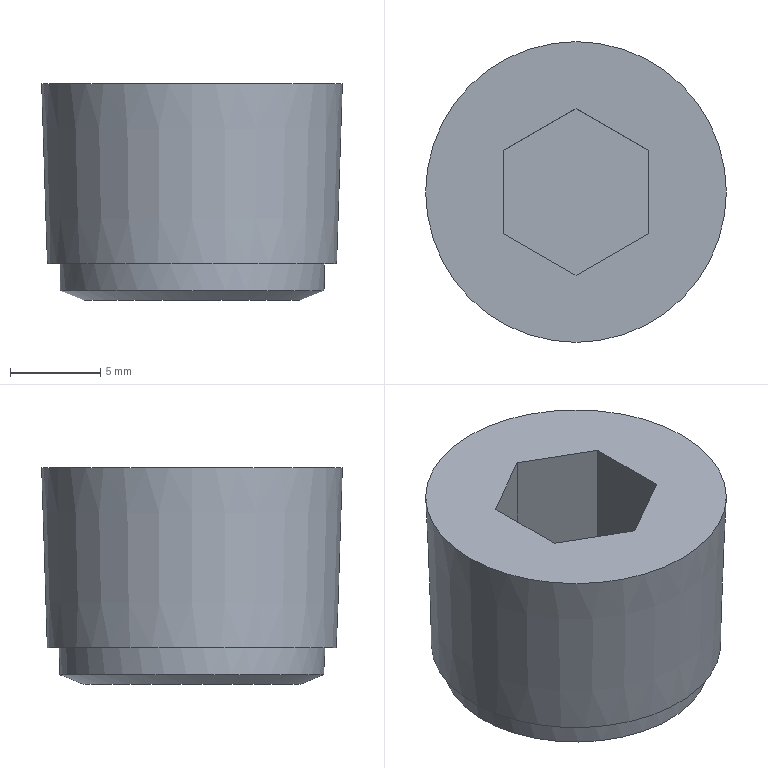Part | STEP file | SOLID | 1 solid | 13 faces | box 16.662 x 16.662 x 12.01 mm | volume 2091 mm3 | plane 10 | cone 3
STEP:
#1=CARTESIAN_POINT('',(0.,0.,0.));
#2=DIRECTION('',(0.,0.,1.));
#3=DIRECTION('',(1.,0.,0.));
#4=AXIS2_PLACEMENT_3D('',#1,#2,#3);
#5=CARTESIAN_POINT('',(0.,8.331,0.));
#6=VERTEX_POINT('',#5);
#7=CARTESIAN_POINT('',(0.,0.,0.));
#8=DIRECTION('',(0.,0.,1.));
#9=DIRECTION('',(0.,1.,0.));
#10=AXIS2_PLACEMENT_3D('',#7,#8,#9);
#11=CIRCLE('',#10,8.331);
#12=CARTESIAN_POINT('',(0.,0.,0.));
#13=DIRECTION('',(0.,0.,1.));
#14=DIRECTION('',(0.,1.,0.));
#15=AXIS2_PLACEMENT_3D('',#12,#13,#14);
#16=PLANE('',#15);
#17=CARTESIAN_POINT('',(0.,0.));
#18=DIRECTION('',(1.,0.));
#19=AXIS2_PLACEMENT_2D('',#17,#18);
#20=CIRCLE('',#19,8.331);
#21=(GEOMETRIC_REPRESENTATION_CONTEXT(2)PARAMETRIC_REPRESENTATION_CONTEXT()REPRESENTATION_CONTEXT('',''));
#22=DEFINITIONAL_REPRESENTATION('',(#20),#21);
#23=PCURVE('',#16,#22);
#24=CARTESIAN_POINT('',(0.,0.,-9.995));
#25=DIRECTION('',(0.,0.,1.));
#26=DIRECTION('',(0.,1.,0.));
#27=AXIS2_PLACEMENT_3D('',#24,#25,#26);
#28=CONICAL_SURFACE('',#27,8.017,0.03142);
#29=CARTESIAN_POINT('',(0.,9.995));
#30=DIRECTION('',(1.,0.));
#31=VECTOR('',#30,1.);
#32=LINE('',#29,#31);
#33=(GEOMETRIC_REPRESENTATION_CONTEXT(2)PARAMETRIC_REPRESENTATION_CONTEXT()REPRESENTATION_CONTEXT('',''));
#34=DEFINITIONAL_REPRESENTATION('',(#32),#33);
#35=PCURVE('',#28,#34);
#36=SURFACE_CURVE('',#11,(#23,#35),.PCURVE_S1.);
#37=EDGE_CURVE('',#6,#6,#36,.T.);
#38=ORIENTED_EDGE('',*,*,#37,.T.);
#39=EDGE_LOOP('',(#38));
#40=FACE_BOUND('',#39,.T.);
#41=CARTESIAN_POINT('',(-4.,-2.309,0.));
#42=VERTEX_POINT('',#41);
#43=CARTESIAN_POINT('',(-4.,2.309,0.));
#44=VERTEX_POINT('',#43);
#45=CARTESIAN_POINT('',(-4.,0.,0.));
#46=DIRECTION('',(0.,1.,0.));
#47=VECTOR('',#46,1.);
#48=LINE('',#45,#47);
#49=CARTESIAN_POINT('',(0.,4.));
#50=DIRECTION('',(1.,0.));
#51=VECTOR('',#50,1.);
#52=LINE('',#49,#51);
#53=(GEOMETRIC_REPRESENTATION_CONTEXT(2)PARAMETRIC_REPRESENTATION_CONTEXT()REPRESENTATION_CONTEXT('',''));
#54=DEFINITIONAL_REPRESENTATION('',(#52),#53);
#55=PCURVE('',#16,#54);
#56=CARTESIAN_POINT('',(-4.,-2.309,-5.));
#57=DIRECTION('',(1.,0.,0.));
#58=DIRECTION('',(0.,-1.,0.));
#59=AXIS2_PLACEMENT_3D('',#56,#57,#58);
#60=PLANE('',#59);
#61=CARTESIAN_POINT('',(-2.309,-5.));
#62=DIRECTION('',(-1.,0.));
#63=VECTOR('',#62,1.);
#64=LINE('',#61,#63);
#65=(GEOMETRIC_REPRESENTATION_CONTEXT(2)PARAMETRIC_REPRESENTATION_CONTEXT()REPRESENTATION_CONTEXT('',''));
#66=DEFINITIONAL_REPRESENTATION('',(#64),#65);
#67=PCURVE('',#60,#66);
#68=SURFACE_CURVE('',#48,(#55,#67),.PCURVE_S1.);
#69=EDGE_CURVE('',#42,#44,#68,.T.);
#70=ORIENTED_EDGE('',*,*,#69,.T.);
#71=CARTESIAN_POINT('',(0.,4.619,0.));
#72=VERTEX_POINT('',#71);
#73=CARTESIAN_POINT('',(-2.,3.464,0.));
#74=DIRECTION('',(0.866,0.5,0.));
#75=VECTOR('',#74,1.);
#76=LINE('',#73,#75);
#77=CARTESIAN_POINT('',(3.464,2.));
#78=DIRECTION('',(0.5,-0.866));
#79=VECTOR('',#78,1.);
#80=LINE('',#77,#79);
#81=(GEOMETRIC_REPRESENTATION_CONTEXT(2)PARAMETRIC_REPRESENTATION_CONTEXT()REPRESENTATION_CONTEXT('',''));
#82=DEFINITIONAL_REPRESENTATION('',(#80),#81);
#83=PCURVE('',#16,#82);
#84=CARTESIAN_POINT('',(-4.,2.309,-5.));
#85=DIRECTION('',(0.5,-0.866,0.));
#86=DIRECTION('',(-0.866,-0.5,0.));
#87=AXIS2_PLACEMENT_3D('',#84,#85,#86);
#88=PLANE('',#87);
#89=CARTESIAN_POINT('',(-2.309,-5.));
#90=DIRECTION('',(-1.,0.));
#91=VECTOR('',#90,1.);
#92=LINE('',#89,#91);
#93=(GEOMETRIC_REPRESENTATION_CONTEXT(2)PARAMETRIC_REPRESENTATION_CONTEXT()REPRESENTATION_CONTEXT('',''));
#94=DEFINITIONAL_REPRESENTATION('',(#92),#93);
#95=PCURVE('',#88,#94);
#96=SURFACE_CURVE('',#76,(#83,#95),.PCURVE_S1.);
#97=EDGE_CURVE('',#44,#72,#96,.T.);
#98=ORIENTED_EDGE('',*,*,#97,.T.);
#99=CARTESIAN_POINT('',(4.,2.309,0.));
#100=VERTEX_POINT('',#99);
#101=CARTESIAN_POINT('',(2.,3.464,0.));
#102=DIRECTION('',(0.866,-0.5,0.));
#103=VECTOR('',#102,1.);
#104=LINE('',#101,#103);
#105=CARTESIAN_POINT('',(3.464,-2.));
#106=DIRECTION('',(-0.5,-0.866));
#107=VECTOR('',#106,1.);
#108=LINE('',#105,#107);
#109=(GEOMETRIC_REPRESENTATION_CONTEXT(2)PARAMETRIC_REPRESENTATION_CONTEXT()REPRESENTATION_CONTEXT('',''));
#110=DEFINITIONAL_REPRESENTATION('',(#108),#109);
#111=PCURVE('',#16,#110);
#112=CARTESIAN_POINT('',(0.,4.619,-5.));
#113=DIRECTION('',(-0.5,-0.866,0.));
#114=DIRECTION('',(-0.866,0.5,0.));
#115=AXIS2_PLACEMENT_3D('',#112,#113,#114);
#116=PLANE('',#115);
#117=CARTESIAN_POINT('',(-2.309,-5.));
#118=DIRECTION('',(-1.,0.));
#119=VECTOR('',#118,1.);
#120=LINE('',#117,#119);
#121=(GEOMETRIC_REPRESENTATION_CONTEXT(2)PARAMETRIC_REPRESENTATION_CONTEXT()REPRESENTATION_CONTEXT('',''));
#122=DEFINITIONAL_REPRESENTATION('',(#120),#121);
#123=PCURVE('',#116,#122);
#124=SURFACE_CURVE('',#104,(#111,#123),.PCURVE_S1.);
#125=EDGE_CURVE('',#72,#100,#124,.T.);
#126=ORIENTED_EDGE('',*,*,#125,.T.);
#127=CARTESIAN_POINT('',(4.,-2.309,0.));
#128=VERTEX_POINT('',#127);
#129=CARTESIAN_POINT('',(4.,0.,0.));
#130=DIRECTION('',(0.,-1.,0.));
#131=VECTOR('',#130,1.);
#132=LINE('',#129,#131);
#133=CARTESIAN_POINT('',(0.,-4.));
#134=DIRECTION('',(-1.,0.));
#135=VECTOR('',#134,1.);
#136=LINE('',#133,#135);
#137=(GEOMETRIC_REPRESENTATION_CONTEXT(2)PARAMETRIC_REPRESENTATION_CONTEXT()REPRESENTATION_CONTEXT('',''));
#138=DEFINITIONAL_REPRESENTATION('',(#136),#137);
#139=PCURVE('',#16,#138);
#140=CARTESIAN_POINT('',(4.,2.309,-5.));
#141=DIRECTION('',(-1.,0.,0.));
#142=DIRECTION('',(0.,1.,0.));
#143=AXIS2_PLACEMENT_3D('',#140,#141,#142);
#144=PLANE('',#143);
#145=CARTESIAN_POINT('',(-2.309,-5.));
#146=DIRECTION('',(-1.,0.));
#147=VECTOR('',#146,1.);
#148=LINE('',#145,#147);
#149=(GEOMETRIC_REPRESENTATION_CONTEXT(2)PARAMETRIC_REPRESENTATION_CONTEXT()REPRESENTATION_CONTEXT('',''));
#150=DEFINITIONAL_REPRESENTATION('',(#148),#149);
#151=PCURVE('',#144,#150);
#152=SURFACE_CURVE('',#132,(#139,#151),.PCURVE_S1.);
#153=EDGE_CURVE('',#100,#128,#152,.T.);
#154=ORIENTED_EDGE('',*,*,#153,.T.);
#155=CARTESIAN_POINT('',(0.,-4.619,0.));
#156=VERTEX_POINT('',#155);
#157=CARTESIAN_POINT('',(2.,-3.464,0.));
#158=DIRECTION('',(-0.866,-0.5,0.));
#159=VECTOR('',#158,1.);
#160=LINE('',#157,#159);
#161=CARTESIAN_POINT('',(-3.464,-2.));
#162=DIRECTION('',(-0.5,0.866));
#163=VECTOR('',#162,1.);
#164=LINE('',#161,#163);
#165=(GEOMETRIC_REPRESENTATION_CONTEXT(2)PARAMETRIC_REPRESENTATION_CONTEXT()REPRESENTATION_CONTEXT('',''));
#166=DEFINITIONAL_REPRESENTATION('',(#164),#165);
#167=PCURVE('',#16,#166);
#168=CARTESIAN_POINT('',(4.,-2.309,-5.));
#169=DIRECTION('',(-0.5,0.866,0.));
#170=DIRECTION('',(0.866,0.5,0.));
#171=AXIS2_PLACEMENT_3D('',#168,#169,#170);
#172=PLANE('',#171);
#173=CARTESIAN_POINT('',(-2.309,-5.));
#174=DIRECTION('',(-1.,0.));
#175=VECTOR('',#174,1.);
#176=LINE('',#173,#175);
#177=(GEOMETRIC_REPRESENTATION_CONTEXT(2)PARAMETRIC_REPRESENTATION_CONTEXT()REPRESENTATION_CONTEXT('',''));
#178=DEFINITIONAL_REPRESENTATION('',(#176),#177);
#179=PCURVE('',#172,#178);
#180=SURFACE_CURVE('',#160,(#167,#179),.PCURVE_S1.);
#181=EDGE_CURVE('',#128,#156,#180,.T.);
#182=ORIENTED_EDGE('',*,*,#181,.T.);
#183=CARTESIAN_POINT('',(-2.,-3.464,0.));
#184=DIRECTION('',(-0.866,0.5,0.));
#185=VECTOR('',#184,1.);
#186=LINE('',#183,#185);
#187=CARTESIAN_POINT('',(-3.464,2.));
#188=DIRECTION('',(0.5,0.866));
#189=VECTOR('',#188,1.);
#190=LINE('',#187,#189);
#191=(GEOMETRIC_REPRESENTATION_CONTEXT(2)PARAMETRIC_REPRESENTATION_CONTEXT()REPRESENTATION_CONTEXT('',''));
#192=DEFINITIONAL_REPRESENTATION('',(#190),#191);
#193=PCURVE('',#16,#192);
#194=CARTESIAN_POINT('',(0.,-4.619,-5.));
#195=DIRECTION('',(0.5,0.866,0.));
#196=DIRECTION('',(0.866,-0.5,0.));
#197=AXIS2_PLACEMENT_3D('',#194,#195,#196);
#198=PLANE('',#197);
#199=CARTESIAN_POINT('',(-2.309,-5.));
#200=DIRECTION('',(-1.,0.));
#201=VECTOR('',#200,1.);
#202=LINE('',#199,#201);
#203=(GEOMETRIC_REPRESENTATION_CONTEXT(2)PARAMETRIC_REPRESENTATION_CONTEXT()REPRESENTATION_CONTEXT('',''));
#204=DEFINITIONAL_REPRESENTATION('',(#202),#203);
#205=PCURVE('',#198,#204);
#206=SURFACE_CURVE('',#186,(#193,#205),.PCURVE_S1.);
#207=EDGE_CURVE('',#156,#42,#206,.T.);
#208=ORIENTED_EDGE('',*,*,#207,.T.);
#209=EDGE_LOOP('',(#70,#98,#126,#154,#182,#208));
#210=FACE_BOUND('',#209,.T.);
#211=ADVANCED_FACE('',(#40,#210),#16,.T.);
#212=CARTESIAN_POINT('',(0.,7.366,-9.995));
#213=VERTEX_POINT('',#212);
#214=CARTESIAN_POINT('',(0.,0.,-9.995));
#215=DIRECTION('',(0.,0.,1.));
#216=DIRECTION('',(0.,1.,0.));
#217=AXIS2_PLACEMENT_3D('',#214,#215,#216);
#218=CIRCLE('',#217,7.366);
#219=CARTESIAN_POINT('',(0.,0.,-9.995));
#220=DIRECTION('',(0.,0.,1.));
#221=DIRECTION('',(0.,1.,0.));
#222=AXIS2_PLACEMENT_3D('',#219,#220,#221);
#223=PLANE('',#222);
#224=CARTESIAN_POINT('',(0.,0.));
#225=DIRECTION('',(1.,0.));
#226=AXIS2_PLACEMENT_2D('',#224,#225);
#227=CIRCLE('',#226,7.366);
#228=(GEOMETRIC_REPRESENTATION_CONTEXT(2)PARAMETRIC_REPRESENTATION_CONTEXT()REPRESENTATION_CONTEXT('',''));
#229=DEFINITIONAL_REPRESENTATION('',(#227),#228);
#230=PCURVE('',#223,#229);
#231=CARTESIAN_POINT('',(0.,0.,-0.6697));
#232=DIRECTION('',(0.,0.,1.));
#233=DIRECTION('',(0.,1.,0.));
#234=AXIS2_PLACEMENT_3D('',#231,#232,#233);
#235=CONICAL_SURFACE('',#234,7.659,0.03142);
#236=CARTESIAN_POINT('',(0.,-9.325));
#237=DIRECTION('',(1.,0.));
#238=VECTOR('',#237,1.);
#239=LINE('',#236,#238);
#240=(GEOMETRIC_REPRESENTATION_CONTEXT(2)PARAMETRIC_REPRESENTATION_CONTEXT()REPRESENTATION_CONTEXT('',''));
#241=DEFINITIONAL_REPRESENTATION('',(#239),#240);
#242=PCURVE('',#235,#241);
#243=SURFACE_CURVE('',#218,(#230,#242),.PCURVE_S1.);
#244=EDGE_CURVE('',#213,#213,#243,.T.);
#245=ORIENTED_EDGE('',*,*,#244,.T.);
#246=EDGE_LOOP('',(#245));
#247=FACE_BOUND('',#246,.T.);
#248=CARTESIAN_POINT('',(0.,8.017,-9.995));
#249=VERTEX_POINT('',#248);
#250=CARTESIAN_POINT('',(0.,0.,-9.995));
#251=DIRECTION('',(0.,0.,1.));
#252=DIRECTION('',(0.,1.,0.));
#253=AXIS2_PLACEMENT_3D('',#250,#251,#252);
#254=CIRCLE('',#253,8.017);
#255=CARTESIAN_POINT('',(0.,0.));
#256=DIRECTION('',(1.,0.));
#257=AXIS2_PLACEMENT_2D('',#255,#256);
#258=CIRCLE('',#257,8.017);
#259=(GEOMETRIC_REPRESENTATION_CONTEXT(2)PARAMETRIC_REPRESENTATION_CONTEXT()REPRESENTATION_CONTEXT('',''));
#260=DEFINITIONAL_REPRESENTATION('',(#258),#259);
#261=PCURVE('',#223,#260);
#262=CARTESIAN_POINT('',(0.,0.));
#263=DIRECTION('',(1.,0.));
#264=VECTOR('',#263,1.);
#265=LINE('',#262,#264);
#266=(GEOMETRIC_REPRESENTATION_CONTEXT(2)PARAMETRIC_REPRESENTATION_CONTEXT()REPRESENTATION_CONTEXT('',''));
#267=DEFINITIONAL_REPRESENTATION('',(#265),#266);
#268=PCURVE('',#28,#267);
#269=SURFACE_CURVE('',#254,(#261,#268),.PCURVE_S1.);
#270=EDGE_CURVE('',#249,#249,#269,.T.);
#271=ORIENTED_EDGE('',*,*,#270,.F.);
#272=EDGE_LOOP('',(#271));
#273=FACE_BOUND('',#272,.T.);
#274=ADVANCED_FACE('',(#247,#273),#223,.F.);
#275=ORIENTED_EDGE('',*,*,#37,.F.);
#276=CARTESIAN_POINT('',(0.,8.017,-9.995));
#277=CARTESIAN_POINT('',(0.,8.331,0.));
#278=B_SPLINE_CURVE_WITH_KNOTS('',1,(#276,#277),.UNSPECIFIED.,.F.,.F.,(2,2),(0.,10.),.PIECEWISE_BEZIER_KNOTS.);
#279=CARTESIAN_POINT('',(0.,0.));
#280=DIRECTION('',(0.,1.));
#281=VECTOR('',#280,1.);
#282=LINE('',#279,#281);
#283=(GEOMETRIC_REPRESENTATION_CONTEXT(2)PARAMETRIC_REPRESENTATION_CONTEXT()REPRESENTATION_CONTEXT('',''));
#284=DEFINITIONAL_REPRESENTATION('',(#282),#283);
#285=PCURVE('',#28,#284);
#286=CARTESIAN_POINT('',(6.283,0.));
#287=DIRECTION('',(0.,1.));
#288=VECTOR('',#287,1.);
#289=LINE('',#286,#288);
#290=(GEOMETRIC_REPRESENTATION_CONTEXT(2)PARAMETRIC_REPRESENTATION_CONTEXT()REPRESENTATION_CONTEXT('',''));
#291=DEFINITIONAL_REPRESENTATION('',(#289),#290);
#292=PCURVE('',#28,#291);
#293=SEAM_CURVE('',#278,(#285,#292),.PCURVE_S1.);
#294=EDGE_CURVE('',#249,#6,#293,.T.);
#295=ORIENTED_EDGE('',*,*,#294,.F.);
#296=ORIENTED_EDGE('',*,*,#270,.T.);
#297=ORIENTED_EDGE('',*,*,#294,.T.);
#298=EDGE_LOOP('',(#275,#295,#296,#297));
#299=FACE_BOUND('',#298,.T.);
#300=ADVANCED_FACE('',(#299),#28,.T.);
#301=CARTESIAN_POINT('',(0.,7.32,-11.468));
#302=VERTEX_POINT('',#301);
#303=CARTESIAN_POINT('',(0.,0.,-11.468));
#304=DIRECTION('',(0.,0.,1.));
#305=DIRECTION('',(0.,1.,0.));
#306=AXIS2_PLACEMENT_3D('',#303,#304,#305);
#307=CIRCLE('',#306,7.32);
#308=CARTESIAN_POINT('',(0.,-10.799));
#309=DIRECTION('',(1.,0.));
#310=VECTOR('',#309,1.);
#311=LINE('',#308,#310);
#312=(GEOMETRIC_REPRESENTATION_CONTEXT(2)PARAMETRIC_REPRESENTATION_CONTEXT()REPRESENTATION_CONTEXT('',''));
#313=DEFINITIONAL_REPRESENTATION('',(#311),#312);
#314=PCURVE('',#235,#313);
#315=CARTESIAN_POINT('',(0.,0.,-11.468));
#316=DIRECTION('',(0.,0.,1.));
#317=DIRECTION('',(0.,1.,0.));
#318=AXIS2_PLACEMENT_3D('',#315,#316,#317);
#319=CONICAL_SURFACE('',#318,7.32,1.181);
#320=CARTESIAN_POINT('',(0.,0.));
#321=DIRECTION('',(1.,0.));
#322=VECTOR('',#321,1.);
#323=LINE('',#320,#322);
#324=(GEOMETRIC_REPRESENTATION_CONTEXT(2)PARAMETRIC_REPRESENTATION_CONTEXT()REPRESENTATION_CONTEXT('',''));
#325=DEFINITIONAL_REPRESENTATION('',(#323),#324);
#326=PCURVE('',#319,#325);
#327=SURFACE_CURVE('',#307,(#314,#326),.PCURVE_S1.);
#328=EDGE_CURVE('',#302,#302,#327,.T.);
#329=ORIENTED_EDGE('',*,*,#328,.T.);
#330=CARTESIAN_POINT('',(0.,7.32,-11.468));
#331=CARTESIAN_POINT('',(0.,7.366,-9.995));
#332=B_SPLINE_CURVE_WITH_KNOTS('',1,(#330,#331),.UNSPECIFIED.,.F.,.F.,(2,2),(-10.804,-9.33),.PIECEWISE_BEZIER_KNOTS.);
#333=CARTESIAN_POINT('',(6.283,0.));
#334=DIRECTION('',(0.,1.));
#335=VECTOR('',#334,1.);
#336=LINE('',#333,#335);
#337=(GEOMETRIC_REPRESENTATION_CONTEXT(2)PARAMETRIC_REPRESENTATION_CONTEXT()REPRESENTATION_CONTEXT('',''));
#338=DEFINITIONAL_REPRESENTATION('',(#336),#337);
#339=PCURVE('',#235,#338);
#340=CARTESIAN_POINT('',(0.,0.));
#341=DIRECTION('',(0.,1.));
#342=VECTOR('',#341,1.);
#343=LINE('',#340,#342);
#344=(GEOMETRIC_REPRESENTATION_CONTEXT(2)PARAMETRIC_REPRESENTATION_CONTEXT()REPRESENTATION_CONTEXT('',''));
#345=DEFINITIONAL_REPRESENTATION('',(#343),#344);
#346=PCURVE('',#235,#345);
#347=SEAM_CURVE('',#332,(#339,#346),.PCURVE_S1.);
#348=EDGE_CURVE('',#302,#213,#347,.T.);
#349=ORIENTED_EDGE('',*,*,#348,.T.);
#350=ORIENTED_EDGE('',*,*,#244,.F.);
#351=ORIENTED_EDGE('',*,*,#348,.F.);
#352=EDGE_LOOP('',(#329,#349,#350,#351));
#353=FACE_BOUND('',#352,.T.);
#354=ADVANCED_FACE('',(#353),#235,.T.);
#355=CARTESIAN_POINT('',(0.,6.,-12.01));
#356=VERTEX_POINT('',#355);
#357=CARTESIAN_POINT('',(0.,0.,-12.01));
#358=DIRECTION('',(0.,0.,1.));
#359=DIRECTION('',(0.,1.,0.));
#360=AXIS2_PLACEMENT_3D('',#357,#358,#359);
#361=CIRCLE('',#360,6.);
#362=CARTESIAN_POINT('',(0.,0.,-12.01));
#363=DIRECTION('',(0.,0.,1.));
#364=DIRECTION('',(0.,1.,0.));
#365=AXIS2_PLACEMENT_3D('',#362,#363,#364);
#366=PLANE('',#365);
#367=CARTESIAN_POINT('',(0.,0.));
#368=DIRECTION('',(1.,0.));
#369=AXIS2_PLACEMENT_2D('',#367,#368);
#370=CIRCLE('',#369,6.);
#371=(GEOMETRIC_REPRESENTATION_CONTEXT(2)PARAMETRIC_REPRESENTATION_CONTEXT()REPRESENTATION_CONTEXT('',''));
#372=DEFINITIONAL_REPRESENTATION('',(#370),#371);
#373=PCURVE('',#366,#372);
#374=CARTESIAN_POINT('',(0.,-0.5417));
#375=DIRECTION('',(1.,0.));
#376=VECTOR('',#375,1.);
#377=LINE('',#374,#376);
#378=(GEOMETRIC_REPRESENTATION_CONTEXT(2)PARAMETRIC_REPRESENTATION_CONTEXT()REPRESENTATION_CONTEXT('',''));
#379=DEFINITIONAL_REPRESENTATION('',(#377),#378);
#380=PCURVE('',#319,#379);
#381=SURFACE_CURVE('',#361,(#373,#380),.PCURVE_S1.);
#382=EDGE_CURVE('',#356,#356,#381,.T.);
#383=ORIENTED_EDGE('',*,*,#382,.F.);
#384=EDGE_LOOP('',(#383));
#385=FACE_BOUND('',#384,.T.);
#386=ADVANCED_FACE('',(#385),#366,.F.);
#387=ORIENTED_EDGE('',*,*,#382,.T.);
#388=CARTESIAN_POINT('',(0.,6.,-12.01));
#389=CARTESIAN_POINT('',(0.,7.32,-11.468));
#390=B_SPLINE_CURVE_WITH_KNOTS('',1,(#388,#389),.UNSPECIFIED.,.F.,.F.,(2,2),(-1.427,0.),.PIECEWISE_BEZIER_KNOTS.);
#391=CARTESIAN_POINT('',(6.283,0.));
#392=DIRECTION('',(0.,1.));
#393=VECTOR('',#392,1.);
#394=LINE('',#391,#393);
#395=(GEOMETRIC_REPRESENTATION_CONTEXT(2)PARAMETRIC_REPRESENTATION_CONTEXT()REPRESENTATION_CONTEXT('',''));
#396=DEFINITIONAL_REPRESENTATION('',(#394),#395);
#397=PCURVE('',#319,#396);
#398=CARTESIAN_POINT('',(0.,0.));
#399=DIRECTION('',(0.,1.));
#400=VECTOR('',#399,1.);
#401=LINE('',#398,#400);
#402=(GEOMETRIC_REPRESENTATION_CONTEXT(2)PARAMETRIC_REPRESENTATION_CONTEXT()REPRESENTATION_CONTEXT('',''));
#403=DEFINITIONAL_REPRESENTATION('',(#401),#402);
#404=PCURVE('',#319,#403);
#405=SEAM_CURVE('',#390,(#397,#404),.PCURVE_S1.);
#406=EDGE_CURVE('',#356,#302,#405,.T.);
#407=ORIENTED_EDGE('',*,*,#406,.T.);
#408=ORIENTED_EDGE('',*,*,#328,.F.);
#409=ORIENTED_EDGE('',*,*,#406,.F.);
#410=EDGE_LOOP('',(#387,#407,#408,#409));
#411=FACE_BOUND('',#410,.T.);
#412=ADVANCED_FACE('',(#411),#319,.T.);
#413=CARTESIAN_POINT('',(-4.,2.309,-6.));
#414=VERTEX_POINT('',#413);
#415=CARTESIAN_POINT('',(-4.,2.309,-5.));
#416=DIRECTION('',(0.,0.,1.));
#417=VECTOR('',#416,1.);
#418=LINE('',#415,#417);
#419=CARTESIAN_POINT('',(0.,0.));
#420=DIRECTION('',(0.,-1.));
#421=VECTOR('',#420,1.);
#422=LINE('',#419,#421);
#423=(GEOMETRIC_REPRESENTATION_CONTEXT(2)PARAMETRIC_REPRESENTATION_CONTEXT()REPRESENTATION_CONTEXT('',''));
#424=DEFINITIONAL_REPRESENTATION('',(#422),#423);
#425=PCURVE('',#88,#424);
#426=CARTESIAN_POINT('',(-4.619,0.));
#427=DIRECTION('',(0.,-1.));
#428=VECTOR('',#427,1.);
#429=LINE('',#426,#428);
#430=(GEOMETRIC_REPRESENTATION_CONTEXT(2)PARAMETRIC_REPRESENTATION_CONTEXT()REPRESENTATION_CONTEXT('',''));
#431=DEFINITIONAL_REPRESENTATION('',(#429),#430);
#432=PCURVE('',#60,#431);
#433=SURFACE_CURVE('',#418,(#425,#432),.PCURVE_S1.);
#434=EDGE_CURVE('',#414,#44,#433,.T.);
#435=ORIENTED_EDGE('',*,*,#434,.F.);
#436=CARTESIAN_POINT('',(0.,4.619,-6.));
#437=VERTEX_POINT('',#436);
#438=CARTESIAN_POINT('',(-4.,2.309,-6.));
#439=CARTESIAN_POINT('',(-2.667,3.079,-6.));
#440=CARTESIAN_POINT('',(-1.333,3.849,-6.));
#441=CARTESIAN_POINT('',(0.,4.619,-6.));
#442=B_SPLINE_CURVE_WITH_KNOTS('',3,(#438,#439,#440,#441),.UNSPECIFIED.,.F.,.F.,(4,4),(0.,1.),.PIECEWISE_BEZIER_KNOTS.);
#443=CARTESIAN_POINT('',(0.,1.));
#444=CARTESIAN_POINT('',(-1.54,1.));
#445=CARTESIAN_POINT('',(-3.079,1.));
#446=CARTESIAN_POINT('',(-4.619,1.));
#447=B_SPLINE_CURVE_WITH_KNOTS('',3,(#443,#444,#445,#446),.UNSPECIFIED.,.F.,.F.,(4,4),(0.,1.),.PIECEWISE_BEZIER_KNOTS.);
#448=(GEOMETRIC_REPRESENTATION_CONTEXT(2)PARAMETRIC_REPRESENTATION_CONTEXT()REPRESENTATION_CONTEXT('',''));
#449=DEFINITIONAL_REPRESENTATION('',(#447),#448);
#450=PCURVE('',#88,#449);
#451=CARTESIAN_POINT('',(-2.,3.464,-6.));
#452=DIRECTION('',(0.,0.,1.));
#453=DIRECTION('',(0.,1.,0.));
#454=AXIS2_PLACEMENT_3D('',#451,#452,#453);
#455=PLANE('',#454);
#456=CARTESIAN_POINT('',(-1.155,2.));
#457=CARTESIAN_POINT('',(-0.3849,0.6667));
#458=CARTESIAN_POINT('',(0.3849,-0.6667));
#459=CARTESIAN_POINT('',(1.155,-2.));
#460=B_SPLINE_CURVE_WITH_KNOTS('',3,(#456,#457,#458,#459),.UNSPECIFIED.,.F.,.F.,(4,4),(0.,1.),.PIECEWISE_BEZIER_KNOTS.);
#461=(GEOMETRIC_REPRESENTATION_CONTEXT(2)PARAMETRIC_REPRESENTATION_CONTEXT()REPRESENTATION_CONTEXT('',''));
#462=DEFINITIONAL_REPRESENTATION('',(#460),#461);
#463=PCURVE('',#455,#462);
#464=SURFACE_CURVE('',#442,(#450,#463),.PCURVE_S1.);
#465=EDGE_CURVE('',#414,#437,#464,.T.);
#466=ORIENTED_EDGE('',*,*,#465,.T.);
#467=CARTESIAN_POINT('',(0.,4.619,-5.));
#468=DIRECTION('',(0.,0.,1.));
#469=VECTOR('',#468,1.);
#470=LINE('',#467,#469);
#471=CARTESIAN_POINT('',(-4.619,0.));
#472=DIRECTION('',(0.,-1.));
#473=VECTOR('',#472,1.);
#474=LINE('',#471,#473);
#475=(GEOMETRIC_REPRESENTATION_CONTEXT(2)PARAMETRIC_REPRESENTATION_CONTEXT()REPRESENTATION_CONTEXT('',''));
#476=DEFINITIONAL_REPRESENTATION('',(#474),#475);
#477=PCURVE('',#88,#476);
#478=CARTESIAN_POINT('',(0.,0.));
#479=DIRECTION('',(0.,-1.));
#480=VECTOR('',#479,1.);
#481=LINE('',#478,#480);
#482=(GEOMETRIC_REPRESENTATION_CONTEXT(2)PARAMETRIC_REPRESENTATION_CONTEXT()REPRESENTATION_CONTEXT('',''));
#483=DEFINITIONAL_REPRESENTATION('',(#481),#482);
#484=PCURVE('',#116,#483);
#485=SURFACE_CURVE('',#470,(#477,#484),.PCURVE_S1.);
#486=EDGE_CURVE('',#437,#72,#485,.T.);
#487=ORIENTED_EDGE('',*,*,#486,.T.);
#488=ORIENTED_EDGE('',*,*,#97,.F.);
#489=EDGE_LOOP('',(#435,#466,#487,#488));
#490=FACE_BOUND('',#489,.T.);
#491=ADVANCED_FACE('',(#490),#88,.T.);
#492=ORIENTED_EDGE('',*,*,#486,.F.);
#493=CARTESIAN_POINT('',(4.,2.309,-6.));
#494=VERTEX_POINT('',#493);
#495=CARTESIAN_POINT('',(0.,4.619,-6.));
#496=CARTESIAN_POINT('',(1.333,3.849,-6.));
#497=CARTESIAN_POINT('',(2.667,3.079,-6.));
#498=CARTESIAN_POINT('',(4.,2.309,-6.));
#499=B_SPLINE_CURVE_WITH_KNOTS('',3,(#495,#496,#497,#498),.UNSPECIFIED.,.F.,.F.,(4,4),(0.,1.),.PIECEWISE_BEZIER_KNOTS.);
#500=CARTESIAN_POINT('',(0.,1.));
#501=CARTESIAN_POINT('',(-1.54,1.));
#502=CARTESIAN_POINT('',(-3.079,1.));
#503=CARTESIAN_POINT('',(-4.619,1.));
#504=B_SPLINE_CURVE_WITH_KNOTS('',3,(#500,#501,#502,#503),.UNSPECIFIED.,.F.,.F.,(4,4),(0.,1.),.PIECEWISE_BEZIER_KNOTS.);
#505=(GEOMETRIC_REPRESENTATION_CONTEXT(2)PARAMETRIC_REPRESENTATION_CONTEXT()REPRESENTATION_CONTEXT('',''));
#506=DEFINITIONAL_REPRESENTATION('',(#504),#505);
#507=PCURVE('',#116,#506);
#508=CARTESIAN_POINT('',(1.155,-2.));
#509=CARTESIAN_POINT('',(0.3849,-3.333));
#510=CARTESIAN_POINT('',(-0.3849,-4.667));
#511=CARTESIAN_POINT('',(-1.155,-6.));
#512=B_SPLINE_CURVE_WITH_KNOTS('',3,(#508,#509,#510,#511),.UNSPECIFIED.,.F.,.F.,(4,4),(0.,1.),.PIECEWISE_BEZIER_KNOTS.);
#513=(GEOMETRIC_REPRESENTATION_CONTEXT(2)PARAMETRIC_REPRESENTATION_CONTEXT()REPRESENTATION_CONTEXT('',''));
#514=DEFINITIONAL_REPRESENTATION('',(#512),#513);
#515=PCURVE('',#455,#514);
#516=SURFACE_CURVE('',#499,(#507,#515),.PCURVE_S1.);
#517=EDGE_CURVE('',#437,#494,#516,.T.);
#518=ORIENTED_EDGE('',*,*,#517,.T.);
#519=CARTESIAN_POINT('',(4.,2.309,-5.));
#520=DIRECTION('',(0.,0.,1.));
#521=VECTOR('',#520,1.);
#522=LINE('',#519,#521);
#523=CARTESIAN_POINT('',(-4.619,0.));
#524=DIRECTION('',(0.,-1.));
#525=VECTOR('',#524,1.);
#526=LINE('',#523,#525);
#527=(GEOMETRIC_REPRESENTATION_CONTEXT(2)PARAMETRIC_REPRESENTATION_CONTEXT()REPRESENTATION_CONTEXT('',''));
#528=DEFINITIONAL_REPRESENTATION('',(#526),#527);
#529=PCURVE('',#116,#528);
#530=CARTESIAN_POINT('',(0.,0.));
#531=DIRECTION('',(0.,-1.));
#532=VECTOR('',#531,1.);
#533=LINE('',#530,#532);
#534=(GEOMETRIC_REPRESENTATION_CONTEXT(2)PARAMETRIC_REPRESENTATION_CONTEXT()REPRESENTATION_CONTEXT('',''));
#535=DEFINITIONAL_REPRESENTATION('',(#533),#534);
#536=PCURVE('',#144,#535);
#537=SURFACE_CURVE('',#522,(#529,#536),.PCURVE_S1.);
#538=EDGE_CURVE('',#494,#100,#537,.T.);
#539=ORIENTED_EDGE('',*,*,#538,.T.);
#540=ORIENTED_EDGE('',*,*,#125,.F.);
#541=EDGE_LOOP('',(#492,#518,#539,#540));
#542=FACE_BOUND('',#541,.T.);
#543=ADVANCED_FACE('',(#542),#116,.T.);
#544=ORIENTED_EDGE('',*,*,#538,.F.);
#545=CARTESIAN_POINT('',(4.,-2.309,-6.));
#546=VERTEX_POINT('',#545);
#547=CARTESIAN_POINT('',(4.,2.309,-6.));
#548=CARTESIAN_POINT('',(4.,0.7698,-6.));
#549=CARTESIAN_POINT('',(4.,-0.7698,-6.));
#550=CARTESIAN_POINT('',(4.,-2.309,-6.));
#551=B_SPLINE_CURVE_WITH_KNOTS('',3,(#547,#548,#549,#550),.UNSPECIFIED.,.F.,.F.,(4,4),(0.,1.),.PIECEWISE_BEZIER_KNOTS.);
#552=CARTESIAN_POINT('',(0.,1.));
#553=CARTESIAN_POINT('',(-1.54,1.));
#554=CARTESIAN_POINT('',(-3.079,1.));
#555=CARTESIAN_POINT('',(-4.619,1.));
#556=B_SPLINE_CURVE_WITH_KNOTS('',3,(#552,#553,#554,#555),.UNSPECIFIED.,.F.,.F.,(4,4),(0.,1.),.PIECEWISE_BEZIER_KNOTS.);
#557=(GEOMETRIC_REPRESENTATION_CONTEXT(2)PARAMETRIC_REPRESENTATION_CONTEXT()REPRESENTATION_CONTEXT('',''));
#558=DEFINITIONAL_REPRESENTATION('',(#556),#557);
#559=PCURVE('',#144,#558);
#560=CARTESIAN_POINT('',(-1.155,-6.));
#561=CARTESIAN_POINT('',(-2.694,-6.));
#562=CARTESIAN_POINT('',(-4.234,-6.));
#563=CARTESIAN_POINT('',(-5.774,-6.));
#564=B_SPLINE_CURVE_WITH_KNOTS('',3,(#560,#561,#562,#563),.UNSPECIFIED.,.F.,.F.,(4,4),(0.,1.),.PIECEWISE_BEZIER_KNOTS.);
#565=(GEOMETRIC_REPRESENTATION_CONTEXT(2)PARAMETRIC_REPRESENTATION_CONTEXT()REPRESENTATION_CONTEXT('',''));
#566=DEFINITIONAL_REPRESENTATION('',(#564),#565);
#567=PCURVE('',#455,#566);
#568=SURFACE_CURVE('',#551,(#559,#567),.PCURVE_S1.);
#569=EDGE_CURVE('',#494,#546,#568,.T.);
#570=ORIENTED_EDGE('',*,*,#569,.T.);
#571=CARTESIAN_POINT('',(4.,-2.309,-5.));
#572=DIRECTION('',(0.,0.,1.));
#573=VECTOR('',#572,1.);
#574=LINE('',#571,#573);
#575=CARTESIAN_POINT('',(-4.619,0.));
#576=DIRECTION('',(0.,-1.));
#577=VECTOR('',#576,1.);
#578=LINE('',#575,#577);
#579=(GEOMETRIC_REPRESENTATION_CONTEXT(2)PARAMETRIC_REPRESENTATION_CONTEXT()REPRESENTATION_CONTEXT('',''));
#580=DEFINITIONAL_REPRESENTATION('',(#578),#579);
#581=PCURVE('',#144,#580);
#582=CARTESIAN_POINT('',(0.,0.));
#583=DIRECTION('',(0.,-1.));
#584=VECTOR('',#583,1.);
#585=LINE('',#582,#584);
#586=(GEOMETRIC_REPRESENTATION_CONTEXT(2)PARAMETRIC_REPRESENTATION_CONTEXT()REPRESENTATION_CONTEXT('',''));
#587=DEFINITIONAL_REPRESENTATION('',(#585),#586);
#588=PCURVE('',#172,#587);
#589=SURFACE_CURVE('',#574,(#581,#588),.PCURVE_S1.);
#590=EDGE_CURVE('',#546,#128,#589,.T.);
#591=ORIENTED_EDGE('',*,*,#590,.T.);
#592=ORIENTED_EDGE('',*,*,#153,.F.);
#593=EDGE_LOOP('',(#544,#570,#591,#592));
#594=FACE_BOUND('',#593,.T.);
#595=ADVANCED_FACE('',(#594),#144,.T.);
#596=ORIENTED_EDGE('',*,*,#590,.F.);
#597=CARTESIAN_POINT('',(0.,-4.619,-6.));
#598=VERTEX_POINT('',#597);
#599=CARTESIAN_POINT('',(4.,-2.309,-6.));
#600=CARTESIAN_POINT('',(2.667,-3.079,-6.));
#601=CARTESIAN_POINT('',(1.333,-3.849,-6.));
#602=CARTESIAN_POINT('',(0.,-4.619,-6.));
#603=B_SPLINE_CURVE_WITH_KNOTS('',3,(#599,#600,#601,#602),.UNSPECIFIED.,.F.,.F.,(4,4),(0.,1.),.PIECEWISE_BEZIER_KNOTS.);
#604=CARTESIAN_POINT('',(0.,1.));
#605=CARTESIAN_POINT('',(-1.54,1.));
#606=CARTESIAN_POINT('',(-3.079,1.));
#607=CARTESIAN_POINT('',(-4.619,1.));
#608=B_SPLINE_CURVE_WITH_KNOTS('',3,(#604,#605,#606,#607),.UNSPECIFIED.,.F.,.F.,(4,4),(0.,1.),.PIECEWISE_BEZIER_KNOTS.);
#609=(GEOMETRIC_REPRESENTATION_CONTEXT(2)PARAMETRIC_REPRESENTATION_CONTEXT()REPRESENTATION_CONTEXT('',''));
#610=DEFINITIONAL_REPRESENTATION('',(#608),#609);
#611=PCURVE('',#172,#610);
#612=CARTESIAN_POINT('',(-5.774,-6.));
#613=CARTESIAN_POINT('',(-6.543,-4.667));
#614=CARTESIAN_POINT('',(-7.313,-3.333));
#615=CARTESIAN_POINT('',(-8.083,-2.));
#616=B_SPLINE_CURVE_WITH_KNOTS('',3,(#612,#613,#614,#615),.UNSPECIFIED.,.F.,.F.,(4,4),(0.,1.),.PIECEWISE_BEZIER_KNOTS.);
#617=(GEOMETRIC_REPRESENTATION_CONTEXT(2)PARAMETRIC_REPRESENTATION_CONTEXT()REPRESENTATION_CONTEXT('',''));
#618=DEFINITIONAL_REPRESENTATION('',(#616),#617);
#619=PCURVE('',#455,#618);
#620=SURFACE_CURVE('',#603,(#611,#619),.PCURVE_S1.);
#621=EDGE_CURVE('',#546,#598,#620,.T.);
#622=ORIENTED_EDGE('',*,*,#621,.T.);
#623=CARTESIAN_POINT('',(0.,-4.619,-5.));
#624=DIRECTION('',(0.,0.,1.));
#625=VECTOR('',#624,1.);
#626=LINE('',#623,#625);
#627=CARTESIAN_POINT('',(-4.619,0.));
#628=DIRECTION('',(0.,-1.));
#629=VECTOR('',#628,1.);
#630=LINE('',#627,#629);
#631=(GEOMETRIC_REPRESENTATION_CONTEXT(2)PARAMETRIC_REPRESENTATION_CONTEXT()REPRESENTATION_CONTEXT('',''));
#632=DEFINITIONAL_REPRESENTATION('',(#630),#631);
#633=PCURVE('',#172,#632);
#634=CARTESIAN_POINT('',(0.,0.));
#635=DIRECTION('',(0.,-1.));
#636=VECTOR('',#635,1.);
#637=LINE('',#634,#636);
#638=(GEOMETRIC_REPRESENTATION_CONTEXT(2)PARAMETRIC_REPRESENTATION_CONTEXT()REPRESENTATION_CONTEXT('',''));
#639=DEFINITIONAL_REPRESENTATION('',(#637),#638);
#640=PCURVE('',#198,#639);
#641=SURFACE_CURVE('',#626,(#633,#640),.PCURVE_S1.);
#642=EDGE_CURVE('',#598,#156,#641,.T.);
#643=ORIENTED_EDGE('',*,*,#642,.T.);
#644=ORIENTED_EDGE('',*,*,#181,.F.);
#645=EDGE_LOOP('',(#596,#622,#643,#644));
#646=FACE_BOUND('',#645,.T.);
#647=ADVANCED_FACE('',(#646),#172,.T.);
#648=ORIENTED_EDGE('',*,*,#642,.F.);
#649=CARTESIAN_POINT('',(-4.,-2.309,-6.));
#650=VERTEX_POINT('',#649);
#651=CARTESIAN_POINT('',(0.,-4.619,-6.));
#652=CARTESIAN_POINT('',(-1.333,-3.849,-6.));
#653=CARTESIAN_POINT('',(-2.667,-3.079,-6.));
#654=CARTESIAN_POINT('',(-4.,-2.309,-6.));
#655=B_SPLINE_CURVE_WITH_KNOTS('',3,(#651,#652,#653,#654),.UNSPECIFIED.,.F.,.F.,(4,4),(0.,1.),.PIECEWISE_BEZIER_KNOTS.);
#656=CARTESIAN_POINT('',(0.,1.));
#657=CARTESIAN_POINT('',(-1.54,1.));
#658=CARTESIAN_POINT('',(-3.079,1.));
#659=CARTESIAN_POINT('',(-4.619,1.));
#660=B_SPLINE_CURVE_WITH_KNOTS('',3,(#656,#657,#658,#659),.UNSPECIFIED.,.F.,.F.,(4,4),(0.,1.),.PIECEWISE_BEZIER_KNOTS.);
#661=(GEOMETRIC_REPRESENTATION_CONTEXT(2)PARAMETRIC_REPRESENTATION_CONTEXT()REPRESENTATION_CONTEXT('',''));
#662=DEFINITIONAL_REPRESENTATION('',(#660),#661);
#663=PCURVE('',#198,#662);
#664=CARTESIAN_POINT('',(-8.083,-2.));
#665=CARTESIAN_POINT('',(-7.313,-0.6667));
#666=CARTESIAN_POINT('',(-6.543,0.6667));
#667=CARTESIAN_POINT('',(-5.774,2.));
#668=B_SPLINE_CURVE_WITH_KNOTS('',3,(#664,#665,#666,#667),.UNSPECIFIED.,.F.,.F.,(4,4),(0.,1.),.PIECEWISE_BEZIER_KNOTS.);
#669=(GEOMETRIC_REPRESENTATION_CONTEXT(2)PARAMETRIC_REPRESENTATION_CONTEXT()REPRESENTATION_CONTEXT('',''));
#670=DEFINITIONAL_REPRESENTATION('',(#668),#669);
#671=PCURVE('',#455,#670);
#672=SURFACE_CURVE('',#655,(#663,#671),.PCURVE_S1.);
#673=EDGE_CURVE('',#598,#650,#672,.T.);
#674=ORIENTED_EDGE('',*,*,#673,.T.);
#675=CARTESIAN_POINT('',(-4.,-2.309,-5.));
#676=DIRECTION('',(0.,0.,1.));
#677=VECTOR('',#676,1.);
#678=LINE('',#675,#677);
#679=CARTESIAN_POINT('',(-4.619,0.));
#680=DIRECTION('',(0.,-1.));
#681=VECTOR('',#680,1.);
#682=LINE('',#679,#681);
#683=(GEOMETRIC_REPRESENTATION_CONTEXT(2)PARAMETRIC_REPRESENTATION_CONTEXT()REPRESENTATION_CONTEXT('',''));
#684=DEFINITIONAL_REPRESENTATION('',(#682),#683);
#685=PCURVE('',#198,#684);
#686=CARTESIAN_POINT('',(0.,0.));
#687=DIRECTION('',(0.,-1.));
#688=VECTOR('',#687,1.);
#689=LINE('',#686,#688);
#690=(GEOMETRIC_REPRESENTATION_CONTEXT(2)PARAMETRIC_REPRESENTATION_CONTEXT()REPRESENTATION_CONTEXT('',''));
#691=DEFINITIONAL_REPRESENTATION('',(#689),#690);
#692=PCURVE('',#60,#691);
#693=SURFACE_CURVE('',#678,(#685,#692),.PCURVE_S1.);
#694=EDGE_CURVE('',#650,#42,#693,.T.);
#695=ORIENTED_EDGE('',*,*,#694,.T.);
#696=ORIENTED_EDGE('',*,*,#207,.F.);
#697=EDGE_LOOP('',(#648,#674,#695,#696));
#698=FACE_BOUND('',#697,.T.);
#699=ADVANCED_FACE('',(#698),#198,.T.);
#700=ORIENTED_EDGE('',*,*,#694,.F.);
#701=CARTESIAN_POINT('',(-4.,-2.309,-6.));
#702=CARTESIAN_POINT('',(-4.,-0.7698,-6.));
#703=CARTESIAN_POINT('',(-4.,0.7698,-6.));
#704=CARTESIAN_POINT('',(-4.,2.309,-6.));
#705=B_SPLINE_CURVE_WITH_KNOTS('',3,(#701,#702,#703,#704),.UNSPECIFIED.,.F.,.F.,(4,4),(0.,1.),.PIECEWISE_BEZIER_KNOTS.);
#706=CARTESIAN_POINT('',(0.,1.));
#707=CARTESIAN_POINT('',(-1.54,1.));
#708=CARTESIAN_POINT('',(-3.079,1.));
#709=CARTESIAN_POINT('',(-4.619,1.));
#710=B_SPLINE_CURVE_WITH_KNOTS('',3,(#706,#707,#708,#709),.UNSPECIFIED.,.F.,.F.,(4,4),(0.,1.),.PIECEWISE_BEZIER_KNOTS.);
#711=(GEOMETRIC_REPRESENTATION_CONTEXT(2)PARAMETRIC_REPRESENTATION_CONTEXT()REPRESENTATION_CONTEXT('',''));
#712=DEFINITIONAL_REPRESENTATION('',(#710),#711);
#713=PCURVE('',#60,#712);
#714=CARTESIAN_POINT('',(-5.774,2.));
#715=CARTESIAN_POINT('',(-4.234,2.));
#716=CARTESIAN_POINT('',(-2.694,2.));
#717=CARTESIAN_POINT('',(-1.155,2.));
#718=B_SPLINE_CURVE_WITH_KNOTS('',3,(#714,#715,#716,#717),.UNSPECIFIED.,.F.,.F.,(4,4),(0.,1.),.PIECEWISE_BEZIER_KNOTS.);
#719=(GEOMETRIC_REPRESENTATION_CONTEXT(2)PARAMETRIC_REPRESENTATION_CONTEXT()REPRESENTATION_CONTEXT('',''));
#720=DEFINITIONAL_REPRESENTATION('',(#718),#719);
#721=PCURVE('',#455,#720);
#722=SURFACE_CURVE('',#705,(#713,#721),.PCURVE_S1.);
#723=EDGE_CURVE('',#650,#414,#722,.T.);
#724=ORIENTED_EDGE('',*,*,#723,.T.);
#725=ORIENTED_EDGE('',*,*,#434,.T.);
#726=ORIENTED_EDGE('',*,*,#69,.F.);
#727=EDGE_LOOP('',(#700,#724,#725,#726));
#728=FACE_BOUND('',#727,.T.);
#729=ADVANCED_FACE('',(#728),#60,.T.);
#730=ORIENTED_EDGE('',*,*,#465,.F.);
#731=ORIENTED_EDGE('',*,*,#723,.F.);
#732=ORIENTED_EDGE('',*,*,#673,.F.);
#733=ORIENTED_EDGE('',*,*,#621,.F.);
#734=ORIENTED_EDGE('',*,*,#569,.F.);
#735=ORIENTED_EDGE('',*,*,#517,.F.);
#736=EDGE_LOOP('',(#730,#731,#732,#733,#734,#735));
#737=FACE_BOUND('',#736,.T.);
#738=ADVANCED_FACE('',(#737),#455,.T.);
#739=CLOSED_SHELL('',(#211,#274,#300,#354,#386,#412,#491,#543,#595,#647,#699,#729,#738));
#740=MANIFOLD_SOLID_BREP('',#739);
#741=(LENGTH_UNIT()NAMED_UNIT(*)SI_UNIT(.MILLI.,.METRE.));
#742=UNCERTAINTY_MEASURE_WITH_UNIT(LENGTH_MEASURE(0.000002),#741,'','');
#743=(NAMED_UNIT(*)PLANE_ANGLE_UNIT()SI_UNIT($,.RADIAN.));
#744=(NAMED_UNIT(*)SI_UNIT($,.STERADIAN.)SOLID_ANGLE_UNIT());
#745=(GEOMETRIC_REPRESENTATION_CONTEXT(3)GLOBAL_UNCERTAINTY_ASSIGNED_CONTEXT((#742))GLOBAL_UNIT_ASSIGNED_CONTEXT((#741,#743,#744))REPRESENTATION_CONTEXT('',''));
#746=ADVANCED_BREP_SHAPE_REPRESENTATION('',(#4,#740),#745);